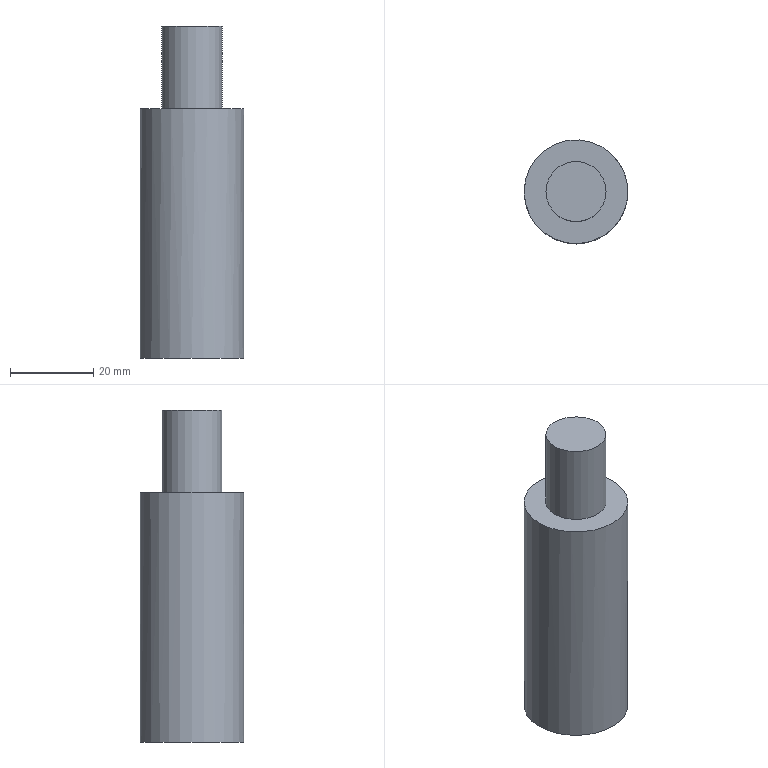Part | NX | features solid 2 | 1 solid | 7 faces | box 25 x 25 x 80 mm | volume 29928 mm3 | plane 4 | cylinder 3 | commonest cylinder face diameters 12 x1 14.5 x1 25 x1
STEP:
#1=CARTESIAN_POINT('',(-572.5,20.,-62.));
#2=VERTEX_POINT('',#1);
#3=CARTESIAN_POINT('',(-560.,20.,-62.));
#4=DIRECTION('',(0.,0.,-1.));
#5=DIRECTION('',(-1.,0.,0.));
#6=AXIS2_PLACEMENT_3D('',#3,#4,#5);
#7=CIRCLE('',#6,12.5);
#8=EDGE_CURVE('',#2,#2,#7,.F.);
#9=ORIENTED_EDGE('',*,*,#8,.F.);
#10=EDGE_LOOP('',(#9));
#11=FACE_BOUND('',#10,.T.);
#12=CARTESIAN_POINT('',(-547.5,20.,-122.));
#13=VERTEX_POINT('',#12);
#14=CARTESIAN_POINT('',(-560.,20.,-122.));
#15=DIRECTION('',(0.,0.,1.));
#16=DIRECTION('',(1.,0.,0.));
#17=AXIS2_PLACEMENT_3D('',#14,#15,#16);
#18=CIRCLE('',#17,12.5);
#19=EDGE_CURVE('',#13,#13,#18,.T.);
#20=ORIENTED_EDGE('',*,*,#19,.T.);
#21=EDGE_LOOP('',(#20));
#22=FACE_BOUND('',#21,.T.);
#23=CARTESIAN_POINT('',(-560.,20.,-22.));
#24=DIRECTION('',(0.,0.,-1.));
#25=DIRECTION('',(-1.,0.,0.));
#26=AXIS2_PLACEMENT_3D('',#23,#24,#25);
#27=CYLINDRICAL_SURFACE('',#26,12.5);
#28=ADVANCED_FACE('',(#11,#22),#27,.T.);
#29=CARTESIAN_POINT('',(-560.,26.,-122.));
#30=VERTEX_POINT('',#29);
#31=CARTESIAN_POINT('',(-560.,20.,-122.));
#32=DIRECTION('',(0.,0.,1.));
#33=DIRECTION('',(0.,1.,0.));
#34=AXIS2_PLACEMENT_3D('',#31,#32,#33);
#35=CIRCLE('',#34,6.);
#36=EDGE_CURVE('',#30,#30,#35,.T.);
#37=ORIENTED_EDGE('',*,*,#36,.T.);
#38=EDGE_LOOP('',(#37));
#39=FACE_BOUND('',#38,.T.);
#40=ORIENTED_EDGE('',*,*,#19,.F.);
#41=EDGE_LOOP('',(#40));
#42=FACE_BOUND('',#41,.T.);
#43=CARTESIAN_POINT('',(-560.,20.,-122.));
#44=DIRECTION('',(0.,0.,1.));
#45=DIRECTION('',(1.,0.,0.));
#46=AXIS2_PLACEMENT_3D('',#43,#44,#45);
#47=PLANE('',#46);
#48=ADVANCED_FACE('',(#39,#42),#47,.F.);
#49=ORIENTED_EDGE('',*,*,#36,.F.);
#50=EDGE_LOOP('',(#49));
#51=FACE_BOUND('',#50,.T.);
#52=CARTESIAN_POINT('',(-560.,26.,-97.));
#53=VERTEX_POINT('',#52);
#54=CARTESIAN_POINT('',(-560.,20.,-97.));
#55=DIRECTION('',(0.,0.,1.));
#56=DIRECTION('',(0.,1.,0.));
#57=AXIS2_PLACEMENT_3D('',#54,#55,#56);
#58=CIRCLE('',#57,6.);
#59=EDGE_CURVE('',#53,#53,#58,.T.);
#60=ORIENTED_EDGE('',*,*,#59,.T.);
#61=EDGE_LOOP('',(#60));
#62=FACE_BOUND('',#61,.T.);
#63=CARTESIAN_POINT('',(-560.,20.,-122.));
#64=DIRECTION('',(0.,0.,1.));
#65=DIRECTION('',(1.,0.,0.));
#66=AXIS2_PLACEMENT_3D('',#63,#64,#65);
#67=CYLINDRICAL_SURFACE('',#66,6.);
#68=ADVANCED_FACE('',(#51,#62),#67,.F.);
#69=ORIENTED_EDGE('',*,*,#59,.F.);
#70=EDGE_LOOP('',(#69));
#71=FACE_BOUND('',#70,.T.);
#72=CARTESIAN_POINT('',(-560.,20.,-97.));
#73=DIRECTION('',(0.,0.,1.));
#74=DIRECTION('',(1.,0.,0.));
#75=AXIS2_PLACEMENT_3D('',#72,#73,#74);
#76=PLANE('',#75);
#77=ADVANCED_FACE('',(#71),#76,.F.);
#78=CARTESIAN_POINT('',(-552.75,20.,-42.));
#79=VERTEX_POINT('',#78);
#80=CARTESIAN_POINT('',(-560.,20.,-42.));
#81=DIRECTION('',(0.,0.,1.));
#82=DIRECTION('',(1.,0.,0.));
#83=AXIS2_PLACEMENT_3D('',#80,#81,#82);
#84=CIRCLE('',#83,7.25);
#85=EDGE_CURVE('',#79,#79,#84,.T.);
#86=ORIENTED_EDGE('',*,*,#85,.F.);
#87=EDGE_LOOP('',(#86));
#88=FACE_BOUND('',#87,.T.);
#89=CARTESIAN_POINT('',(-567.25,20.,-62.));
#90=VERTEX_POINT('',#89);
#91=CARTESIAN_POINT('',(-560.,20.,-62.));
#92=DIRECTION('',(0.,0.,-1.));
#93=DIRECTION('',(-1.,0.,0.));
#94=AXIS2_PLACEMENT_3D('',#91,#92,#93);
#95=CIRCLE('',#94,7.25);
#96=EDGE_CURVE('',#90,#90,#95,.F.);
#97=ORIENTED_EDGE('',*,*,#96,.T.);
#98=EDGE_LOOP('',(#97));
#99=FACE_BOUND('',#98,.T.);
#100=CARTESIAN_POINT('',(-560.,20.,-62.));
#101=DIRECTION('',(0.,0.,1.));
#102=DIRECTION('',(1.,0.,0.));
#103=AXIS2_PLACEMENT_3D('',#100,#101,#102);
#104=CYLINDRICAL_SURFACE('',#103,7.25);
#105=ADVANCED_FACE('',(#88,#99),#104,.T.);
#106=ORIENTED_EDGE('',*,*,#96,.F.);
#107=EDGE_LOOP('',(#106));
#108=FACE_BOUND('',#107,.T.);
#109=ORIENTED_EDGE('',*,*,#8,.T.);
#110=EDGE_LOOP('',(#109));
#111=FACE_BOUND('',#110,.T.);
#112=CARTESIAN_POINT('',(-560.,20.,-62.));
#113=DIRECTION('',(0.,0.,-1.));
#114=DIRECTION('',(-1.,0.,0.));
#115=AXIS2_PLACEMENT_3D('',#112,#113,#114);
#116=PLANE('',#115);
#117=ADVANCED_FACE('',(#108,#111),#116,.F.);
#118=ORIENTED_EDGE('',*,*,#85,.T.);
#119=EDGE_LOOP('',(#118));
#120=FACE_BOUND('',#119,.T.);
#121=CARTESIAN_POINT('',(-560.,20.,-42.));
#122=DIRECTION('',(0.,0.,1.));
#123=DIRECTION('',(1.,0.,0.));
#124=AXIS2_PLACEMENT_3D('',#121,#122,#123);
#125=PLANE('',#124);
#126=ADVANCED_FACE('',(#120),#125,.T.);
#127=CLOSED_SHELL('',(#28,#48,#68,#77,#105,#117,#126));
#128=MANIFOLD_SOLID_BREP('',#127);
#129=(LENGTH_UNIT()NAMED_UNIT(*)SI_UNIT(.MILLI.,.METRE.));
#130=UNCERTAINTY_MEASURE_WITH_UNIT(LENGTH_MEASURE(0.00001),#129,'','');
#131=(NAMED_UNIT(*)PLANE_ANGLE_UNIT()SI_UNIT($,.RADIAN.));
#132=(NAMED_UNIT(*)SI_UNIT($,.STERADIAN.)SOLID_ANGLE_UNIT());
#133=(GEOMETRIC_REPRESENTATION_CONTEXT(3)GLOBAL_UNCERTAINTY_ASSIGNED_CONTEXT((#130))GLOBAL_UNIT_ASSIGNED_CONTEXT((#129,#131,#132))REPRESENTATION_CONTEXT('',''));
#134=ADVANCED_BREP_SHAPE_REPRESENTATION('',(#128),#133);